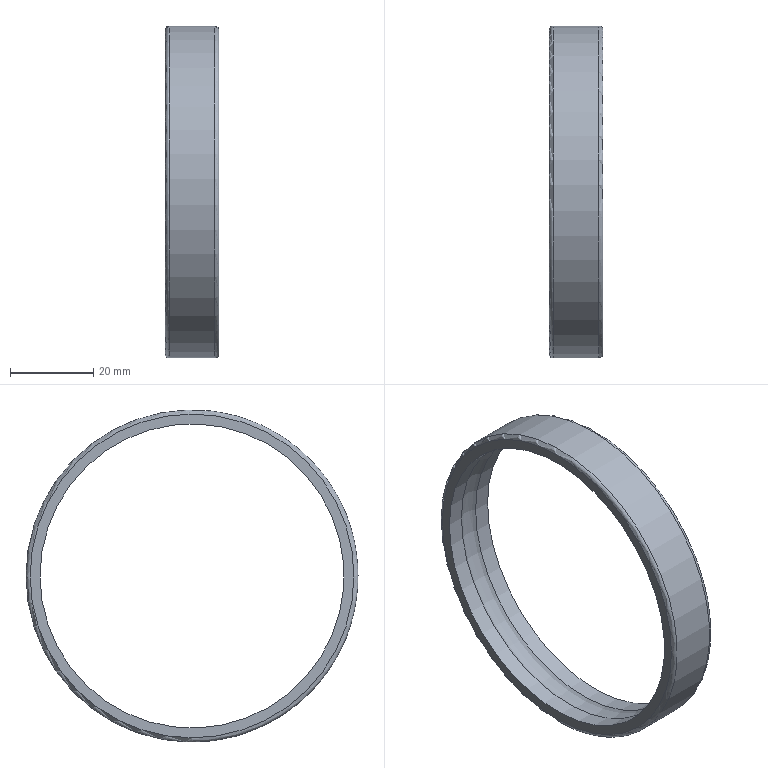Part | STEP file | Outer ring | 1 solid | 8 faces | box 13 x 80 x 80 mm | volume 9785 mm3 | cylinder 3 | torus 3 | plane 2 | commonest cylinder face diameters 73.25 x2 80 x1
STEP:
#1=CARTESIAN_POINT('',(-2.408,36.625,0.));
#2=VERTEX_POINT('',#1);
#3=CARTESIAN_POINT('',(-2.408,0.,0.));
#4=DIRECTION('',(1.,0.,0.));
#5=DIRECTION('',(0.,1.,0.));
#6=AXIS2_PLACEMENT_3D('',#3,#4,#5);
#7=CIRCLE('',#6,36.625);
#8=EDGE_CURVE('',#2,#2,#7,.T.);
#9=ORIENTED_EDGE('',*,*,#8,.T.);
#10=EDGE_LOOP('',(#9));
#11=FACE_OUTER_BOUND('',#10,.T.);
#12=CARTESIAN_POINT('',(-6.5,36.625,0.));
#13=VERTEX_POINT('',#12);
#14=CARTESIAN_POINT('',(-6.5,0.,0.));
#15=DIRECTION('',(1.,0.,0.));
#16=DIRECTION('',(0.,1.,0.));
#17=AXIS2_PLACEMENT_3D('',#14,#15,#16);
#18=CIRCLE('',#17,36.625);
#19=EDGE_CURVE('',#13,#13,#18,.T.);
#20=ORIENTED_EDGE('',*,*,#19,.F.);
#21=EDGE_LOOP('',(#20));
#22=FACE_OUTER_BOUND('',#21,.T.);
#23=CARTESIAN_POINT('',(6.5,0.,0.));
#24=DIRECTION('',(1.,0.,0.));
#25=DIRECTION('',(0.,1.,0.));
#26=AXIS2_PLACEMENT_3D('',#23,#24,#25);
#27=CYLINDRICAL_SURFACE('',#26,36.625);
#28=ADVANCED_FACE('',(#11,#22),#27,.F.);
#29=CARTESIAN_POINT('',(6.5,36.625,0.));
#30=VERTEX_POINT('',#29);
#31=CARTESIAN_POINT('',(6.5,0.,0.));
#32=DIRECTION('',(1.,0.,0.));
#33=DIRECTION('',(0.,1.,0.));
#34=AXIS2_PLACEMENT_3D('',#31,#32,#33);
#35=CIRCLE('',#34,36.625);
#36=EDGE_CURVE('',#30,#30,#35,.T.);
#37=ORIENTED_EDGE('',*,*,#36,.T.);
#38=EDGE_LOOP('',(#37));
#39=FACE_OUTER_BOUND('',#38,.T.);
#40=CARTESIAN_POINT('',(2.408,36.625,0.));
#41=VERTEX_POINT('',#40);
#42=CARTESIAN_POINT('',(2.408,0.,0.));
#43=DIRECTION('',(1.,0.,0.));
#44=DIRECTION('',(0.,1.,0.));
#45=AXIS2_PLACEMENT_3D('',#42,#43,#44);
#46=CIRCLE('',#45,36.625);
#47=EDGE_CURVE('',#41,#41,#46,.F.);
#48=ORIENTED_EDGE('',*,*,#47,.T.);
#49=EDGE_LOOP('',(#48));
#50=FACE_OUTER_BOUND('',#49,.T.);
#51=CARTESIAN_POINT('',(6.5,0.,0.));
#52=DIRECTION('',(1.,0.,0.));
#53=DIRECTION('',(0.,1.,0.));
#54=AXIS2_PLACEMENT_3D('',#51,#52,#53);
#55=CYLINDRICAL_SURFACE('',#54,36.625);
#56=ADVANCED_FACE('',(#39,#50),#55,.F.);
#57=ORIENTED_EDGE('',*,*,#47,.F.);
#58=EDGE_LOOP('',(#57));
#59=FACE_OUTER_BOUND('',#58,.T.);
#60=ORIENTED_EDGE('',*,*,#8,.F.);
#61=EDGE_LOOP('',(#60));
#62=FACE_OUTER_BOUND('',#61,.T.);
#63=CARTESIAN_POINT('',(0.,0.,0.));
#64=DIRECTION('',(1.,0.,0.));
#65=DIRECTION('',(0.,1.,0.));
#66=AXIS2_PLACEMENT_3D('',#63,#64,#65);
#67=TOROIDAL_SURFACE('',#66,33.75,3.75);
#68=ADVANCED_FACE('',(#59,#62),#67,.F.);
#69=CARTESIAN_POINT('',(-6.5,39.,0.));
#70=VERTEX_POINT('',#69);
#71=CARTESIAN_POINT('',(-6.5,0.,0.));
#72=DIRECTION('',(1.,0.,0.));
#73=DIRECTION('',(0.,1.,0.));
#74=AXIS2_PLACEMENT_3D('',#71,#72,#73);
#75=CIRCLE('',#74,39.);
#76=EDGE_CURVE('',#70,#70,#75,.T.);
#77=ORIENTED_EDGE('',*,*,#76,.F.);
#78=EDGE_LOOP('',(#77));
#79=FACE_BOUND('',#78,.T.);
#80=ORIENTED_EDGE('',*,*,#19,.T.);
#81=EDGE_LOOP('',(#80));
#82=FACE_BOUND('',#81,.T.);
#83=CARTESIAN_POINT('',(-6.5,0.,0.));
#84=DIRECTION('',(-1.,0.,0.));
#85=DIRECTION('',(0.,1.,0.));
#86=AXIS2_PLACEMENT_3D('',#83,#84,#85);
#87=PLANE('',#86);
#88=ADVANCED_FACE('',(#79,#82),#87,.T.);
#89=CARTESIAN_POINT('',(6.5,39.,0.));
#90=VERTEX_POINT('',#89);
#91=CARTESIAN_POINT('',(6.5,0.,0.));
#92=DIRECTION('',(1.,0.,0.));
#93=DIRECTION('',(0.,1.,0.));
#94=AXIS2_PLACEMENT_3D('',#91,#92,#93);
#95=CIRCLE('',#94,39.);
#96=EDGE_CURVE('',#90,#90,#95,.T.);
#97=ORIENTED_EDGE('',*,*,#96,.T.);
#98=EDGE_LOOP('',(#97));
#99=FACE_BOUND('',#98,.T.);
#100=ORIENTED_EDGE('',*,*,#36,.F.);
#101=EDGE_LOOP('',(#100));
#102=FACE_BOUND('',#101,.T.);
#103=CARTESIAN_POINT('',(6.5,0.,0.));
#104=DIRECTION('',(1.,0.,0.));
#105=DIRECTION('',(0.,1.,0.));
#106=AXIS2_PLACEMENT_3D('',#103,#104,#105);
#107=PLANE('',#106);
#108=ADVANCED_FACE('',(#99,#102),#107,.T.);
#109=CARTESIAN_POINT('',(5.5,40.,0.));
#110=VERTEX_POINT('',#109);
#111=CARTESIAN_POINT('',(5.5,0.,0.));
#112=DIRECTION('',(1.,0.,0.));
#113=DIRECTION('',(0.,1.,0.));
#114=AXIS2_PLACEMENT_3D('',#111,#112,#113);
#115=CIRCLE('',#114,40.);
#116=EDGE_CURVE('',#110,#110,#115,.T.);
#117=ORIENTED_EDGE('',*,*,#116,.F.);
#118=EDGE_LOOP('',(#117));
#119=FACE_OUTER_BOUND('',#118,.T.);
#120=CARTESIAN_POINT('',(-5.5,40.,0.));
#121=VERTEX_POINT('',#120);
#122=CARTESIAN_POINT('',(-5.5,0.,0.));
#123=DIRECTION('',(1.,0.,0.));
#124=DIRECTION('',(0.,1.,0.));
#125=AXIS2_PLACEMENT_3D('',#122,#123,#124);
#126=CIRCLE('',#125,40.);
#127=EDGE_CURVE('',#121,#121,#126,.T.);
#128=ORIENTED_EDGE('',*,*,#127,.T.);
#129=EDGE_LOOP('',(#128));
#130=FACE_OUTER_BOUND('',#129,.T.);
#131=CARTESIAN_POINT('',(-6.5,0.,0.));
#132=DIRECTION('',(1.,0.,0.));
#133=DIRECTION('',(0.,1.,0.));
#134=AXIS2_PLACEMENT_3D('',#131,#132,#133);
#135=CYLINDRICAL_SURFACE('',#134,40.);
#136=ADVANCED_FACE('',(#119,#130),#135,.T.);
#137=ORIENTED_EDGE('',*,*,#127,.F.);
#138=EDGE_LOOP('',(#137));
#139=FACE_OUTER_BOUND('',#138,.T.);
#140=ORIENTED_EDGE('',*,*,#76,.T.);
#141=EDGE_LOOP('',(#140));
#142=FACE_OUTER_BOUND('',#141,.T.);
#143=CARTESIAN_POINT('',(-5.5,0.,0.));
#144=DIRECTION('',(1.,0.,0.));
#145=DIRECTION('',(0.,1.,0.));
#146=AXIS2_PLACEMENT_3D('',#143,#144,#145);
#147=TOROIDAL_SURFACE('',#146,39.,1.);
#148=ADVANCED_FACE('',(#139,#142),#147,.T.);
#149=ORIENTED_EDGE('',*,*,#96,.F.);
#150=EDGE_LOOP('',(#149));
#151=FACE_OUTER_BOUND('',#150,.T.);
#152=ORIENTED_EDGE('',*,*,#116,.T.);
#153=EDGE_LOOP('',(#152));
#154=FACE_OUTER_BOUND('',#153,.T.);
#155=CARTESIAN_POINT('',(5.5,0.,0.));
#156=DIRECTION('',(1.,0.,0.));
#157=DIRECTION('',(0.,1.,0.));
#158=AXIS2_PLACEMENT_3D('',#155,#156,#157);
#159=TOROIDAL_SURFACE('',#158,39.,1.);
#160=ADVANCED_FACE('',(#151,#154),#159,.T.);
#161=CLOSED_SHELL('',(#28,#56,#68,#88,#108,#136,#148,#160));
#162=MANIFOLD_SOLID_BREP('',#161);
#163=(LENGTH_UNIT()NAMED_UNIT(*)SI_UNIT(.MILLI.,.METRE.));
#164=UNCERTAINTY_MEASURE_WITH_UNIT(LENGTH_MEASURE(0.00001),#163,'','');
#165=(NAMED_UNIT(*)PLANE_ANGLE_UNIT()SI_UNIT($,.RADIAN.));
#166=(NAMED_UNIT(*)SI_UNIT($,.STERADIAN.)SOLID_ANGLE_UNIT());
#167=(GEOMETRIC_REPRESENTATION_CONTEXT(3)GLOBAL_UNCERTAINTY_ASSIGNED_CONTEXT((#164))GLOBAL_UNIT_ASSIGNED_CONTEXT((#163,#165,#166))REPRESENTATION_CONTEXT('',''));
#168=ADVANCED_BREP_SHAPE_REPRESENTATION('',(#162),#167);